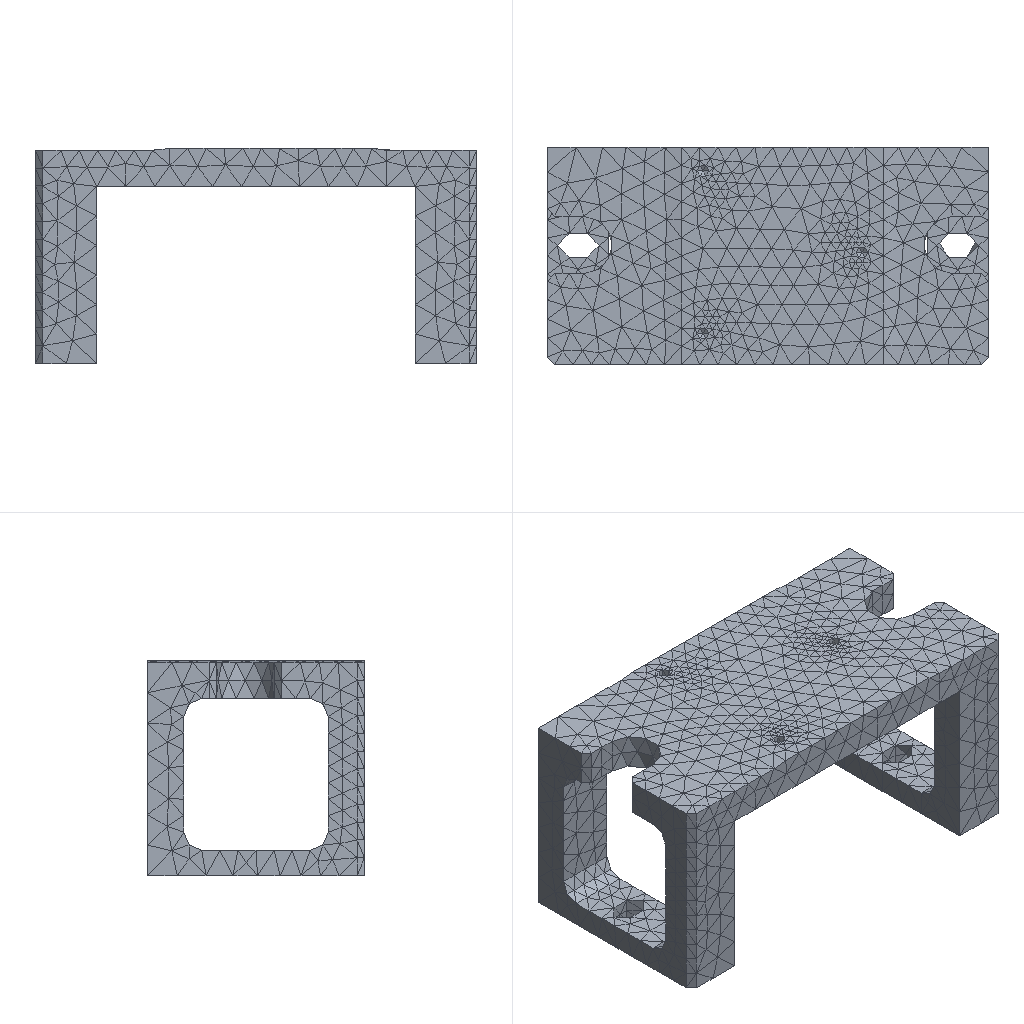Simulation study | nx simcenter
Set-up summary:
category,name,step,type,value,unit,region
solver,nx_nastran (Simcenter)
units,not stated in the deck,,not stated
analysis,deck,,static,static
analysis,solution,,SOL,101
load_step,SUBCASE 1,1,SUBCASE,SPC=1 LOAD=2
load_step,requested,,,1
mesh,nodes,,,7406
mesh,elements,,,3653
element_type,CTETRA,,solid,3653
load,nodal force total,,FX,0.0,model units
load,nodal force total,,FY,0.0,model units
load,nodal force total,,FZ,-1000000.053,model units
load,load commands in deck,,count,656
bc,support commands in deck,,count,256
analysis,NX solution 0,,Structural,Linear Statics - Single Constraint
check,setup vs results,,match,every grid point's frame and coordinates and every element id; grid points of CTETRA elements
Nastran input file, long lists of numbers shortened:
$*$$$$$$$$$$$$$$$$$$$$$$$$$$$$$$$$$$$$$$$$$$$$$$$$$$$$$$$$$$$$$$$$$
$*
$*                    NX v10.0.0.24 TRANSLATOR
$*                    FOR NX NASTRAN VERSION 10.0
$ (33 more lines like these left out)
ASSIGN OUTPUT2='121_sim1-solution_1.op2' UNIT=12
$*
$*$$$$$$$$$$$$$$$$$$$$$$$$$$$$$$$$$$$
$*
$* EXECUTIVE CONTROL
$*
$*$$$$$$$$$$$$$$$$$$$$$$$$$$$$$$$$$$$
$*
ID,NASTRAN,121_sim1-solution_1
SOL 101
CEND
$*
$*$$$$$$$$$$$$$$$$$$$$$$$$$$$$$$$$$$$
$*
$* CASE CONTROL
$*
$*$$$$$$$$$$$$$$$$$$$$$$$$$$$$$$$$$$$
$*
TITLE = Solution 1
ECHO = NONE
SPC = 1
OUTPUT
BCRESULTS(TRACTION,FORCE,PLOT) = ALL
DISPLACEMENT(PLOT) = ALL
ESE(PLOT) = ALL
FORCE(PLOT,CORNER) = ALL
OLOAD(PLOT) = ALL
SPCFORCES(PLOT) = ALL
STRAIN(PLOT,FIBER,CORNER) = ALL
STRESS(PLOT,CORNER) = ALL
$*  NX Step: Subcase - Static Loads 1
SUBCASE 1
LABEL = Subcase - Static Loads 1
LOAD = 2
$*
$*$$$$$$$$$$$$$$$$$$$$$$$$$$$$$$$$$$$
$*
$* BULK DATA
$*
$*$$$$$$$$$$$$$$$$$$$$$$$$$$$$$$$$$$$
$*
BEGIN BULK
$*
$* PARAM CARDS
$*
PARAM      K6ROT100.0000
PARAM     OIBULK     YES
PARAM    OMACHPR     YES
PARAM       POST      -2
PARAM    POSTEXT     YES
PARAM    UNITSYS   MN-MM
$*
$* GRID CARDS
$*
GRID*               7305               0-6.100000000E+012.0000000000E+00+
*       -1.000000000E+00               0
GRID*               7306               0-6.100000000E+012.0000000000E+00+
*       5.8000000000E+01               0
$ (14808 more lines like these left out)
$*
$* ELEMENT CARDS
$*
$*  NX Mesh Collector: Solid(1)
$*  NX Mesh: 3d_mesh(1)
CTETRA         1       1       1    4290    6838       2     109    4747+
+            110     111     112     113
CTETRA         2       1    6735    3547    6684    3291    3767     114+
+            115    3459     116     117
$ (7302 more lines like these left out)
$*
$* PROPERTY CARDS
$*
$*  NX Property: PSOLID1
PSOLID         1       2       0                           SMECH
$*
$* MATERIAL CARDS
$*
$*  NX Material: Aluminum_6061
MAT1           26.8980+7        0.3300002.7110-62.2161-5
MATT1          2       1               2               3
TABLEM1        1                                                        +
+        20.00006.8980+7 21.11006.8980+7 23.89006.8980+7 37.78006.8290+7+
+        51.67006.8290+7 65.56006.7600+7 79.44006.6910+7 93.33006.6221+7+
+       107.22006.5531+7121.11006.4841+7135.00006.4151+7148.89006.3461+7+
+       162.78006.2772+7176.67006.1392+7190.56006.0702+7204.44005.9323+7+
+       218.33005.8633+7232.22005.7253+7246.11005.5874+7260.00005.4494+7+
+       273.89005.3114+7287.78005.1735+7301.67005.0355+7315.56004.8976+7+
+       329.44004.7596+7343.33004.6216+7357.22004.4147+7371.11004.2767+7+
+       385.00004.1388+7398.89003.9318+7412.78003.7939+7426.67003.5869+7+
+           ENDT
TABLEM1        2                                                        +
+        20.00000.330000 21.11000.330000    ENDT
TABLEM1        3                                                        +
+        20.00002.2380-5 93.33002.3184-5107.22002.3346-5121.11002.3508-5+
+       135.00002.3670-5148.89002.3832-5162.78002.3994-5176.67002.4138-5+
+       190.56002.4300-5204.44002.4444-5218.33002.4588-5232.22002.4732-5+
+       246.11002.4876-5260.00002.5002-5273.89002.5146-5287.78002.5272-5+
+       301.67002.5398-5315.56002.5524-5    ENDT
$*
$* LOAD AND CONSTRAINT CARDS
$*
$*  NX Load and Constraint: Fixed(1)
SPC            1    3042  123456  0.0000
SPC            1    3043  123456  0.0000
SPC            1    3044  123456  0.0000
SPC            1    3045  123456  0.0000
$ (252 more lines like these left out)
$*  NX Load and Constraint: Force(1)
FORCE          2    4339       0 1312.07  0.0000  0.0000-1.00000
FORCE          2    4340       0 1476.02  0.0000  0.0000-1.00000
FORCE          2    4341       0980.8241  0.0000  0.0000-1.00000
FORCE          2    4342       0780.8709  0.0000  0.0000-1.00000
$ (652 more lines like these left out)
ENDDATA e89fac15
Results summary:
result,analysis,,,static
result,last_loadstep,,,1
result,primary field,,,displacements
result,reaction total,,FX,-0.006836,model units
result,reaction total,,FY,0.003174,model units
result,reaction total,,FZ,1000000.062,model units
result,NX solution 0,,loadcases,1,mm